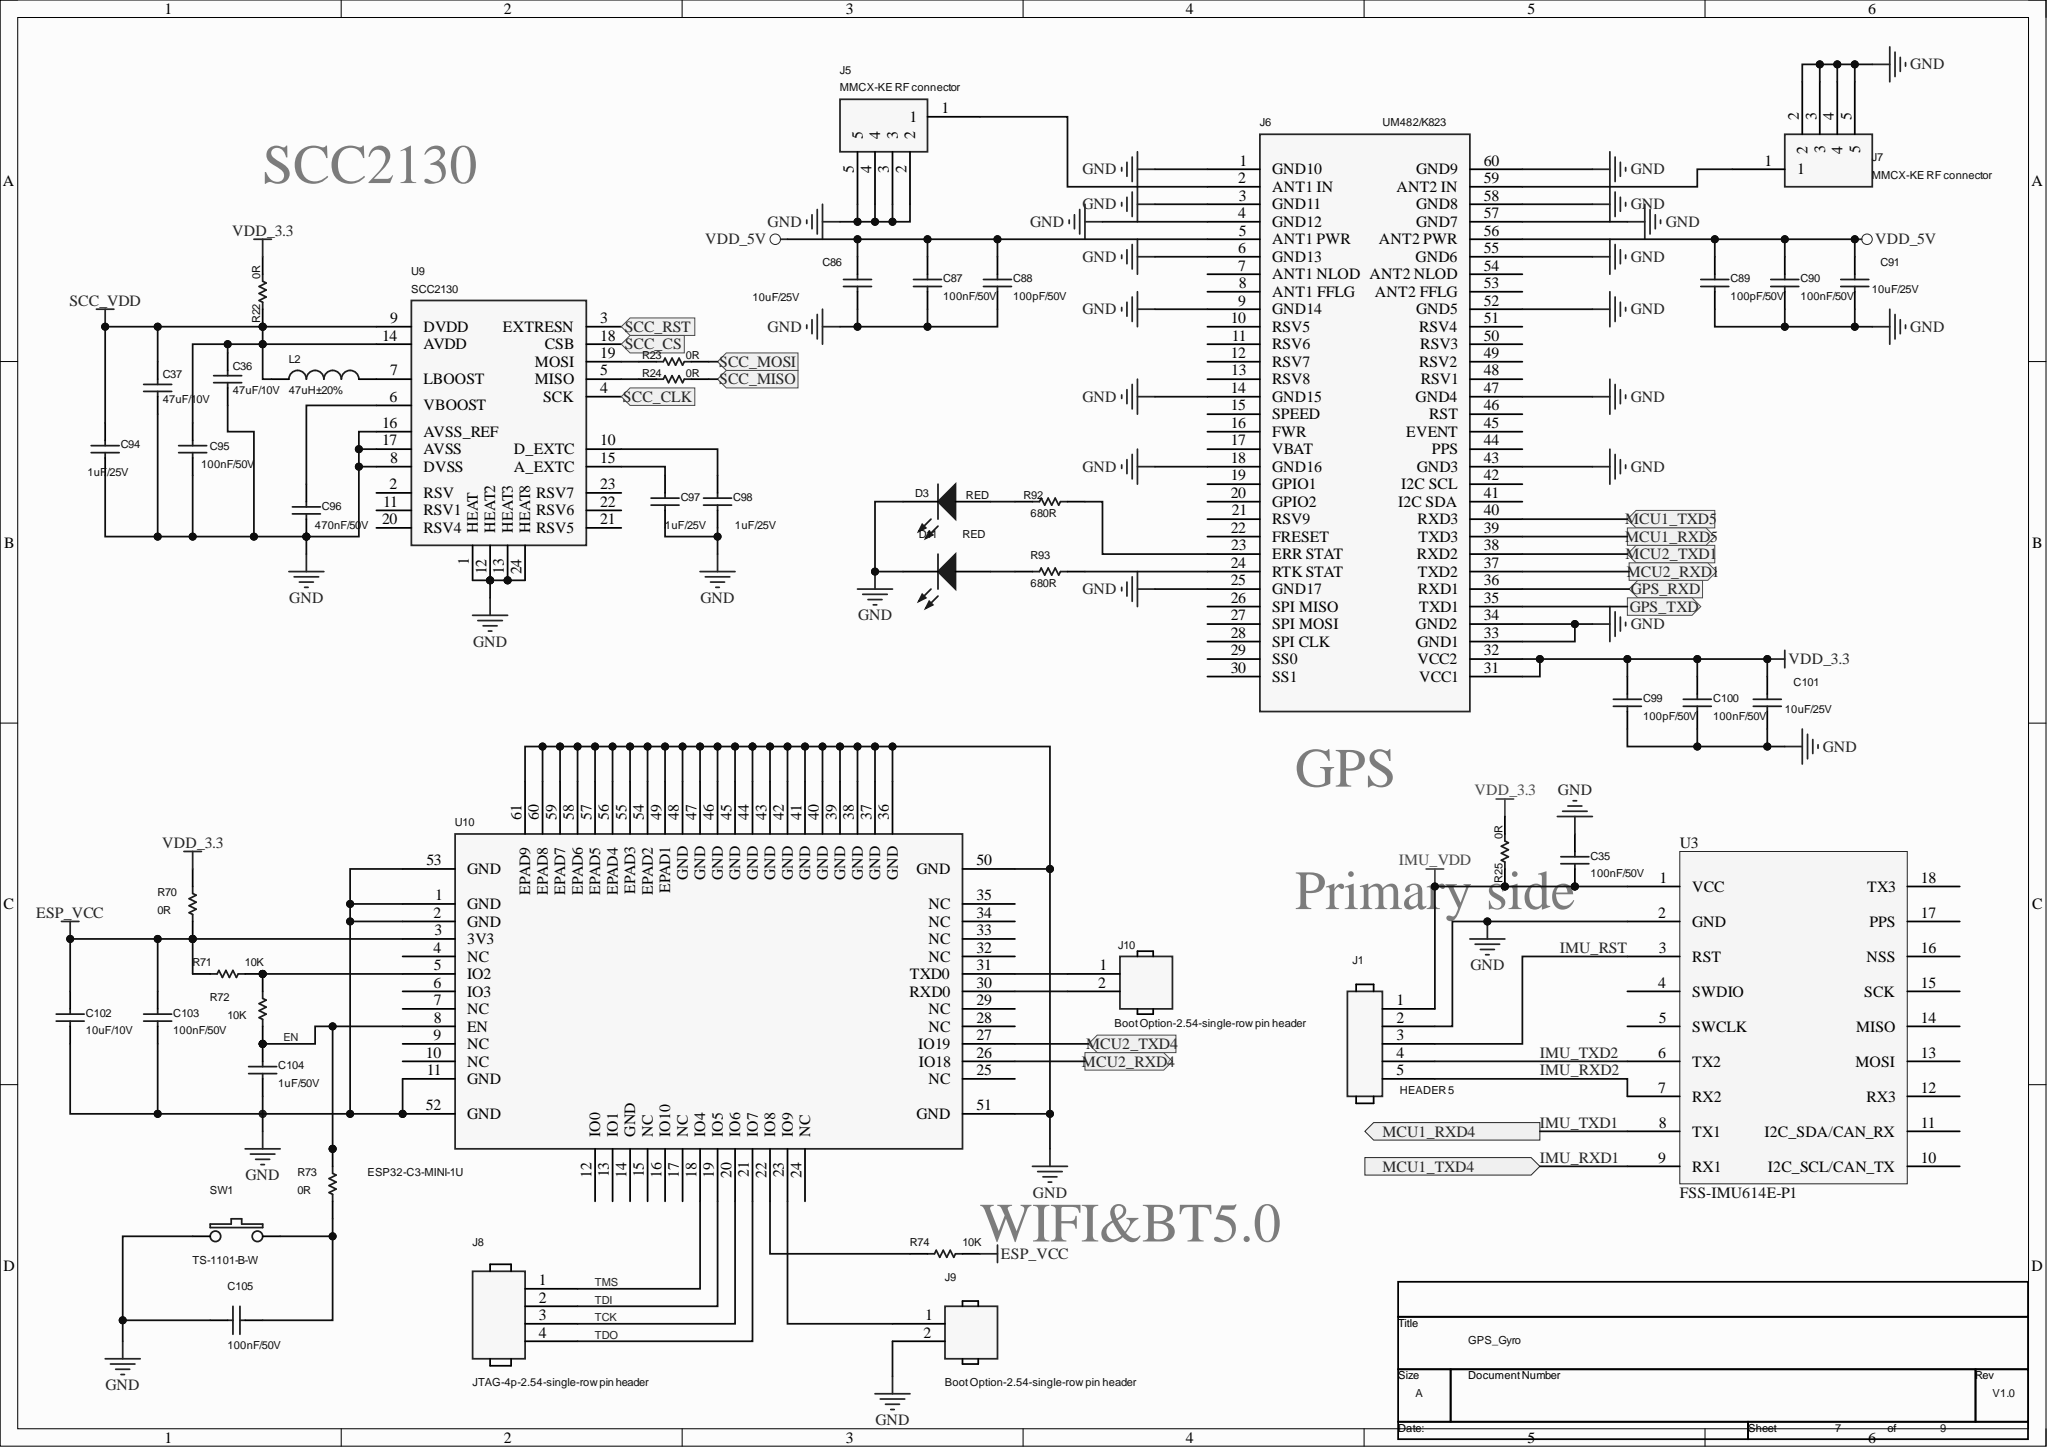Circuit board | Altium Designer | 313 parts | 216 nets | one sheet of the schematic
Parts on this sheet (reference | value | footprint):
C35 | 100nF/50V | 0603
C36 | 47uF/10V | CAP-SMD_L3.5-W2.8
C37 | 47uF/10V | CAP-SMD_L3.5-W2.8
C86 | 10uF/25V | C0805
C87 | 100nF/50V | 0603
C88 | 100pF/50V | 0603
C89 | 100pF/50V | 0603
C90 | 100nF/50V | 0603
C91 | 10uF/25V | C0805
C94 | 1uF/25V | 0603
C95 | 100nF/50V | 0603
C96 | 470nF/50V | 0603
C97 | 1uF/25V | 0603
C98 | 1uF/25V | 0603
C99 | 100pF/50V | 0603
C100 | 100nF/50V | 0603
C101 | 10uF/25V | C0805
C102 | 100nF/50V | C0603
C103 | 100nF/50V | C0603
C104 | 100nF/50V | C0603
C105 | 100nF/50V | C0603
D3 | RED | LED_0805
D11 | RED | LED_0805
J1 | HEADER 5 | 2.54mm_paizhen_5pin
J5 | MMCX-KE RF connector | MMCX-KE
J6 | UM482/K823 | UM482_K823
J7 | MMCX-KE RF connector | MMCX-KE
J8 | JTAG-4p-2.54-single-row pin header | HDR_1X4_254
J9 | Boot Option-2.54-single-row pin header | HDR_1X2_254
J10 | Boot Option-2.54-single-row pin header | HDR_1X2_254
L2 | 47uH±20% | 1210
R22 | 0R | R0603
R23 | 0R | R0603
R24 | 0R | R0603
R25 | 0R | R0603
R70 | 0R | R0603
R71 | 10K | R0603
R72 | 10K | R0603
R73 | 0R | R0603
R74 | 10K | R0603
R92 | NA | 0603
R93 | NA | 0603
SW1 | TS-1101-B-W | SMD
U3 | FSS-IMU614E-P1 | FSS-IMU614E-P1
U9 | SCC2130 | SCC2130D
U10 | ESP32-C3-MINI-1U | WIFIM-SMD_ESP32-C3-MINI-1
Nets of these parts (net: part-pin ...):
VDD_5V: C86-2 C87-1 C88-1 C89-2 C90-2 C91-2 J6-5 J6-56
VDD_3.3: C99-2 C100-2 C101-2 R22-1 R25-1 R70-1 J6-31 J6-32
TMS: J8-1 U10-18
TDO: J8-4 U10-21
TDI: J8-2 U10-19
TCK: J8-3 U10-20
SCC_VDD: C36-1 C37-1 C94-1 C95-1 L2-1 R22-2 U9-9 U9-14
NetU1_44: U9-3
NetU1_41: U9-4
NetU1_40: U9-18
NetR74_2: R74-2 U10-22
NetR71_1: R71-1 R72-1 U10-5
NetR24_2: R24-2 U9-5
NetR24_1: R24-1
NetR23_2: R23-2 U9-19
NetR23_1: R23-1
NetL2_2: L2-2 U9-7
NetJ10_2: J10-2 U10-30
NetJ10_1: J10-1 U10-31
NetJ9_1: J9-1 U10-23
NetJ6_59: J7-1 J6-59
NetJ6_24: R93-1 J6-24
NetJ6_23: R92-1 J6-23
NetJ5_1: J5-1 J6-2
NetD11_1: D11-1 R93-2
NetD3_1: D3-1 R92-2
NetC105_1: C105-1 R73-2 SW1-2
NetC98_1: C98-1 U9-10
NetC97_1: C97-1 U9-15
NetC96_1: C96-1 U9-6
IMU_VDD: C35-1 J1-1 R25-2 U3-1
IMU_TXD2: J1-4 U3-6
IMU_TXD1: U3-8
IMU_RXD2: J1-5 U3-7
IMU_RXD1: U3-9
IMU_RST: J1-3 U3-3
GND: C35-2 C36-2 C37-2 C86-1 C87-2 C88-2 C89-1 C90-1 C91-1 C94-2 C95-2 C96-2 C97-2 C98-2 C99-1 C100-1 C101-1 C102-1 C103-1 C104-1 C105-2 D3-2 D11-2 J1-2 J5-2 J5-3 J5-4 J5-5 J7-2 J7-3 J7-4 J7-5 J9-2 SW1-1 U3-2 U9-1 U9-8 U9-12 U9-13 U9-16 U9-17 U9-24 J6-1 J6-3 J6-4 J6-6 J6-9 J6-14 J6-18 J6-25 J6-33 J6-34 J6-43 J6-47 J6-52 J6-55 J6-57 J6-58 J6-60 U10-1 U10-2 U10-11 U10-36 U10-37 U10-38 U10-39 U10-40 U10-41 U10-42 U10-43 U10-44 U10-45 U10-46 U10-47 U10-48 U10-49 U10-50 U10-51 U10-52 U10-53 U10-54 U10-55 U10-56 U10-57 U10-58 U10-59 U10-60 U10-61
ESP_VCC: C102-2 C103-2 R70-2 R71-2 R74-1 U10-3
EN: C104-2 R72-2 R73-1 U10-8